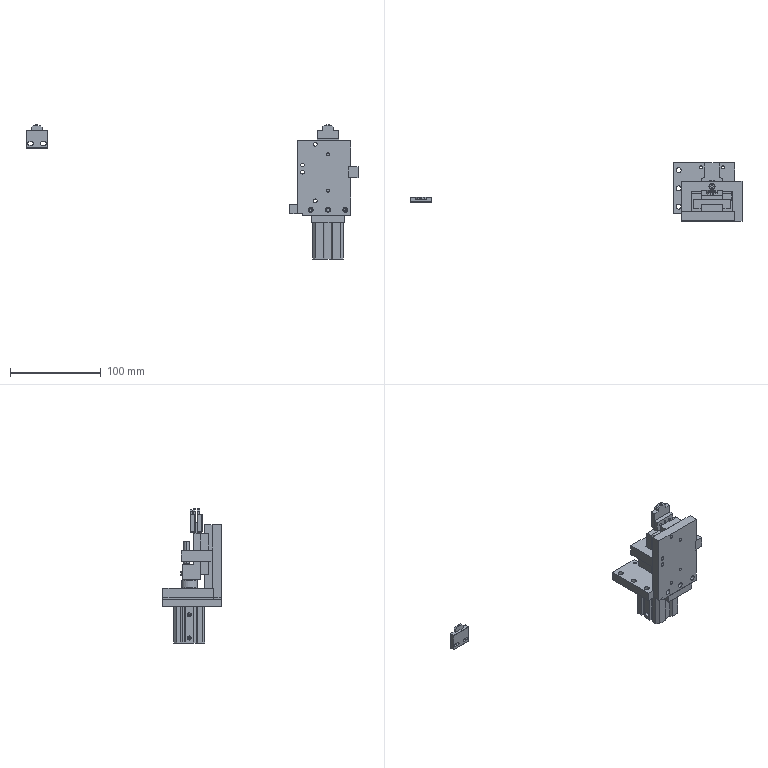Part | NX | 11 solids | 461 faces | box 365 x 64 x 147.34 mm | volume 204273 mm3 | plane 225 | cylinder 163 | cone 72 | sphere 1 | commonest cylinder face diameters 2.5 x20 3.5 x20 4.2 x18 4.5 x16 5.5 x16 6.5 x16